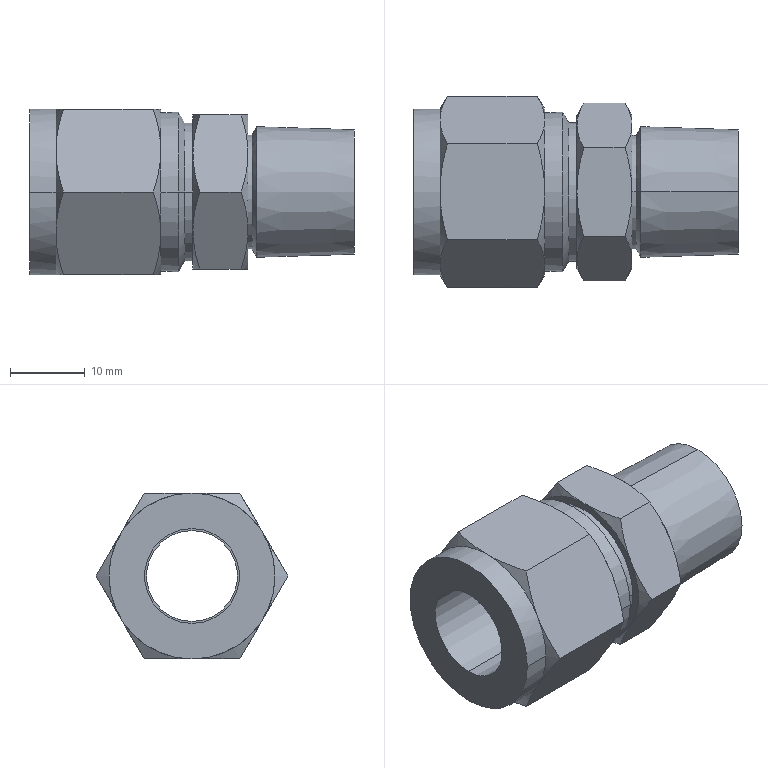Part | STEP file | straight fittingV11_.50 TUBE X .38 NPT | 1 solid | 63 faces | box 43.434 x 25.663 x 22.225 mm | volume 9265 mm3 | cone 32 | plane 19 | cylinder 12 | commonest cylinder face diameters 12.7 x4 12.192 x2 15.268 x2 18.522 x2 22.225 x2